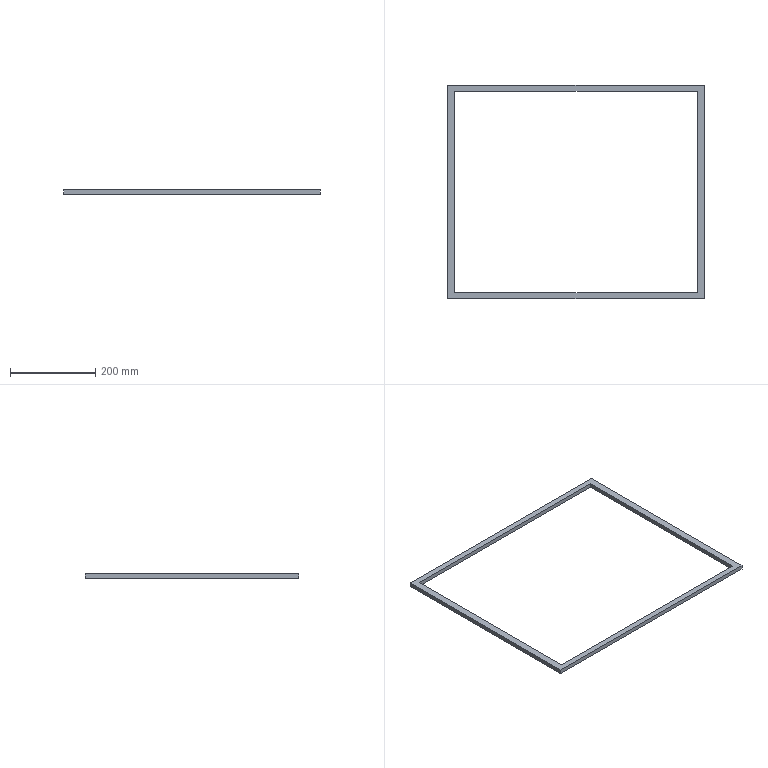Part | SolidWorks | features Extrusion 1 | 1 solid | 10 faces | box 600 x 500 x 10 mm | volume 317236 mm3 | plane 10
STEP:
#1=CARTESIAN_POINT('',(300.,-250.,10.));
#2=VERTEX_POINT('',#1);
#3=CARTESIAN_POINT('',(300.,250.,10.));
#4=VERTEX_POINT('',#3);
#5=CARTESIAN_POINT('',(300.,250.,10.));
#6=DIRECTION('',(0.,1.,0.));
#7=VECTOR('',#6,1000.);
#8=LINE('',#5,#7);
#9=EDGE_CURVE('',#2,#4,#8,.T.);
#10=ORIENTED_EDGE('',*,*,#9,.T.);
#11=CARTESIAN_POINT('',(-300.,250.,10.));
#12=VERTEX_POINT('',#11);
#13=CARTESIAN_POINT('',(-300.,250.,10.));
#14=DIRECTION('',(-1.,0.,0.));
#15=VECTOR('',#14,1000.);
#16=LINE('',#13,#15);
#17=EDGE_CURVE('',#4,#12,#16,.T.);
#18=ORIENTED_EDGE('',*,*,#17,.T.);
#19=CARTESIAN_POINT('',(-300.,-250.,10.));
#20=VERTEX_POINT('',#19);
#21=CARTESIAN_POINT('',(-300.,250.,10.));
#22=DIRECTION('',(0.,-1.,0.));
#23=VECTOR('',#22,1000.);
#24=LINE('',#21,#23);
#25=EDGE_CURVE('',#12,#20,#24,.T.);
#26=ORIENTED_EDGE('',*,*,#25,.T.);
#27=CARTESIAN_POINT('',(-300.,-250.,10.));
#28=DIRECTION('',(1.,0.,0.));
#29=VECTOR('',#28,1000.);
#30=LINE('',#27,#29);
#31=EDGE_CURVE('',#20,#2,#30,.T.);
#32=ORIENTED_EDGE('',*,*,#31,.T.);
#33=EDGE_LOOP('',(#10,#18,#26,#32));
#34=FACE_OUTER_BOUND('',#33,.T.);
#35=CARTESIAN_POINT('',(283.695,236.413,10.));
#36=VERTEX_POINT('',#35);
#37=CARTESIAN_POINT('',(-283.695,236.413,10.));
#38=VERTEX_POINT('',#37);
#39=CARTESIAN_POINT('',(-283.695,236.413,10.));
#40=DIRECTION('',(-1.,0.,0.));
#41=VECTOR('',#40,1000.);
#42=LINE('',#39,#41);
#43=EDGE_CURVE('',#36,#38,#42,.T.);
#44=ORIENTED_EDGE('',*,*,#43,.F.);
#45=CARTESIAN_POINT('',(283.695,-236.413,10.));
#46=VERTEX_POINT('',#45);
#47=CARTESIAN_POINT('',(283.695,236.413,10.));
#48=DIRECTION('',(0.,1.,0.));
#49=VECTOR('',#48,1000.);
#50=LINE('',#47,#49);
#51=EDGE_CURVE('',#46,#36,#50,.T.);
#52=ORIENTED_EDGE('',*,*,#51,.F.);
#53=CARTESIAN_POINT('',(-283.695,-236.413,10.));
#54=VERTEX_POINT('',#53);
#55=CARTESIAN_POINT('',(-283.695,-236.413,10.));
#56=DIRECTION('',(1.,0.,0.));
#57=VECTOR('',#56,1000.);
#58=LINE('',#55,#57);
#59=EDGE_CURVE('',#54,#46,#58,.T.);
#60=ORIENTED_EDGE('',*,*,#59,.F.);
#61=CARTESIAN_POINT('',(-283.695,236.413,10.));
#62=DIRECTION('',(0.,-1.,0.));
#63=VECTOR('',#62,1000.);
#64=LINE('',#61,#63);
#65=EDGE_CURVE('',#38,#54,#64,.T.);
#66=ORIENTED_EDGE('',*,*,#65,.F.);
#67=EDGE_LOOP('',(#44,#52,#60,#66));
#68=FACE_BOUND('',#67,.T.);
#69=CARTESIAN_POINT('',(0.,0.,10.));
#70=DIRECTION('',(0.,0.,1.));
#71=DIRECTION('',(1.,0.,0.));
#72=AXIS2_PLACEMENT_3D('',#69,#70,#71);
#73=PLANE('',#72);
#74=ADVANCED_FACE('',(#34,#68),#73,.T.);
#75=CARTESIAN_POINT('',(300.,-250.,0.));
#76=VERTEX_POINT('',#75);
#77=CARTESIAN_POINT('',(300.,250.,0.));
#78=VERTEX_POINT('',#77);
#79=CARTESIAN_POINT('',(300.,250.,0.));
#80=DIRECTION('',(0.,1.,0.));
#81=VECTOR('',#80,1000.);
#82=LINE('',#79,#81);
#83=EDGE_CURVE('',#76,#78,#82,.T.);
#84=ORIENTED_EDGE('',*,*,#83,.F.);
#85=CARTESIAN_POINT('',(-300.,-250.,0.));
#86=VERTEX_POINT('',#85);
#87=CARTESIAN_POINT('',(-300.,-250.,0.));
#88=DIRECTION('',(1.,0.,0.));
#89=VECTOR('',#88,1000.);
#90=LINE('',#87,#89);
#91=EDGE_CURVE('',#86,#76,#90,.T.);
#92=ORIENTED_EDGE('',*,*,#91,.F.);
#93=CARTESIAN_POINT('',(-300.,250.,0.));
#94=VERTEX_POINT('',#93);
#95=CARTESIAN_POINT('',(-300.,250.,0.));
#96=DIRECTION('',(0.,-1.,0.));
#97=VECTOR('',#96,1000.);
#98=LINE('',#95,#97);
#99=EDGE_CURVE('',#94,#86,#98,.T.);
#100=ORIENTED_EDGE('',*,*,#99,.F.);
#101=CARTESIAN_POINT('',(-300.,250.,0.));
#102=DIRECTION('',(-1.,0.,0.));
#103=VECTOR('',#102,1000.);
#104=LINE('',#101,#103);
#105=EDGE_CURVE('',#78,#94,#104,.T.);
#106=ORIENTED_EDGE('',*,*,#105,.F.);
#107=EDGE_LOOP('',(#84,#92,#100,#106));
#108=FACE_OUTER_BOUND('',#107,.T.);
#109=CARTESIAN_POINT('',(283.695,-236.413,0.));
#110=VERTEX_POINT('',#109);
#111=CARTESIAN_POINT('',(283.695,236.413,0.));
#112=VERTEX_POINT('',#111);
#113=CARTESIAN_POINT('',(283.695,236.413,0.));
#114=DIRECTION('',(0.,1.,0.));
#115=VECTOR('',#114,1000.);
#116=LINE('',#113,#115);
#117=EDGE_CURVE('',#110,#112,#116,.T.);
#118=ORIENTED_EDGE('',*,*,#117,.T.);
#119=CARTESIAN_POINT('',(-283.695,236.413,0.));
#120=VERTEX_POINT('',#119);
#121=CARTESIAN_POINT('',(-283.695,236.413,0.));
#122=DIRECTION('',(-1.,0.,0.));
#123=VECTOR('',#122,1000.);
#124=LINE('',#121,#123);
#125=EDGE_CURVE('',#112,#120,#124,.T.);
#126=ORIENTED_EDGE('',*,*,#125,.T.);
#127=CARTESIAN_POINT('',(-283.695,-236.413,0.));
#128=VERTEX_POINT('',#127);
#129=CARTESIAN_POINT('',(-283.695,236.413,0.));
#130=DIRECTION('',(0.,-1.,0.));
#131=VECTOR('',#130,1000.);
#132=LINE('',#129,#131);
#133=EDGE_CURVE('',#120,#128,#132,.T.);
#134=ORIENTED_EDGE('',*,*,#133,.T.);
#135=CARTESIAN_POINT('',(-283.695,-236.413,0.));
#136=DIRECTION('',(1.,0.,0.));
#137=VECTOR('',#136,1000.);
#138=LINE('',#135,#137);
#139=EDGE_CURVE('',#128,#110,#138,.T.);
#140=ORIENTED_EDGE('',*,*,#139,.T.);
#141=EDGE_LOOP('',(#118,#126,#134,#140));
#142=FACE_BOUND('',#141,.T.);
#143=CARTESIAN_POINT('',(0.,0.,0.));
#144=DIRECTION('',(0.,0.,1.));
#145=DIRECTION('',(1.,0.,0.));
#146=AXIS2_PLACEMENT_3D('',#143,#144,#145);
#147=PLANE('',#146);
#148=ADVANCED_FACE('',(#108,#142),#147,.F.);
#149=ORIENTED_EDGE('',*,*,#83,.T.);
#150=CARTESIAN_POINT('',(300.,250.,10.));
#151=DIRECTION('',(0.,0.,-1.));
#152=VECTOR('',#151,1000.);
#153=LINE('',#150,#152);
#154=EDGE_CURVE('',#4,#78,#153,.T.);
#155=ORIENTED_EDGE('',*,*,#154,.F.);
#156=ORIENTED_EDGE('',*,*,#9,.F.);
#157=CARTESIAN_POINT('',(300.,-250.,10.));
#158=DIRECTION('',(0.,0.,-1.));
#159=VECTOR('',#158,1000.);
#160=LINE('',#157,#159);
#161=EDGE_CURVE('',#2,#76,#160,.T.);
#162=ORIENTED_EDGE('',*,*,#161,.T.);
#163=EDGE_LOOP('',(#149,#155,#156,#162));
#164=FACE_OUTER_BOUND('',#163,.T.);
#165=CARTESIAN_POINT('',(300.,250.,10.));
#166=DIRECTION('',(-1.,0.,0.));
#167=DIRECTION('',(0.,-1.,0.));
#168=AXIS2_PLACEMENT_3D('',#165,#166,#167);
#169=PLANE('',#168);
#170=ADVANCED_FACE('',(#164),#169,.F.);
#171=ORIENTED_EDGE('',*,*,#105,.T.);
#172=CARTESIAN_POINT('',(-300.,250.,10.));
#173=DIRECTION('',(0.,0.,-1.));
#174=VECTOR('',#173,1000.);
#175=LINE('',#172,#174);
#176=EDGE_CURVE('',#12,#94,#175,.T.);
#177=ORIENTED_EDGE('',*,*,#176,.F.);
#178=ORIENTED_EDGE('',*,*,#17,.F.);
#179=ORIENTED_EDGE('',*,*,#154,.T.);
#180=EDGE_LOOP('',(#171,#177,#178,#179));
#181=FACE_OUTER_BOUND('',#180,.T.);
#182=CARTESIAN_POINT('',(-300.,250.,10.));
#183=DIRECTION('',(0.,-1.,0.));
#184=DIRECTION('',(0.,0.,-1.));
#185=AXIS2_PLACEMENT_3D('',#182,#183,#184);
#186=PLANE('',#185);
#187=ADVANCED_FACE('',(#181),#186,.F.);
#188=ORIENTED_EDGE('',*,*,#99,.T.);
#189=CARTESIAN_POINT('',(-300.,-250.,10.));
#190=DIRECTION('',(0.,0.,-1.));
#191=VECTOR('',#190,1000.);
#192=LINE('',#189,#191);
#193=EDGE_CURVE('',#20,#86,#192,.T.);
#194=ORIENTED_EDGE('',*,*,#193,.F.);
#195=ORIENTED_EDGE('',*,*,#25,.F.);
#196=ORIENTED_EDGE('',*,*,#176,.T.);
#197=EDGE_LOOP('',(#188,#194,#195,#196));
#198=FACE_OUTER_BOUND('',#197,.T.);
#199=CARTESIAN_POINT('',(-300.,250.,10.));
#200=DIRECTION('',(1.,0.,0.));
#201=DIRECTION('',(0.,1.,0.));
#202=AXIS2_PLACEMENT_3D('',#199,#200,#201);
#203=PLANE('',#202);
#204=ADVANCED_FACE('',(#198),#203,.F.);
#205=ORIENTED_EDGE('',*,*,#91,.T.);
#206=ORIENTED_EDGE('',*,*,#161,.F.);
#207=ORIENTED_EDGE('',*,*,#31,.F.);
#208=ORIENTED_EDGE('',*,*,#193,.T.);
#209=EDGE_LOOP('',(#205,#206,#207,#208));
#210=FACE_OUTER_BOUND('',#209,.T.);
#211=CARTESIAN_POINT('',(-300.,-250.,10.));
#212=DIRECTION('',(0.,1.,0.));
#213=DIRECTION('',(0.,0.,1.));
#214=AXIS2_PLACEMENT_3D('',#211,#212,#213);
#215=PLANE('',#214);
#216=ADVANCED_FACE('',(#210),#215,.F.);
#217=ORIENTED_EDGE('',*,*,#117,.F.);
#218=CARTESIAN_POINT('',(283.695,-236.413,10.));
#219=DIRECTION('',(0.,0.,-1.));
#220=VECTOR('',#219,1000.);
#221=LINE('',#218,#220);
#222=EDGE_CURVE('',#46,#110,#221,.T.);
#223=ORIENTED_EDGE('',*,*,#222,.F.);
#224=ORIENTED_EDGE('',*,*,#51,.T.);
#225=CARTESIAN_POINT('',(283.695,236.413,10.));
#226=DIRECTION('',(0.,0.,-1.));
#227=VECTOR('',#226,1000.);
#228=LINE('',#225,#227);
#229=EDGE_CURVE('',#36,#112,#228,.T.);
#230=ORIENTED_EDGE('',*,*,#229,.T.);
#231=EDGE_LOOP('',(#217,#223,#224,#230));
#232=FACE_OUTER_BOUND('',#231,.T.);
#233=CARTESIAN_POINT('',(283.695,236.413,10.));
#234=DIRECTION('',(-1.,0.,0.));
#235=DIRECTION('',(0.,0.,1.));
#236=AXIS2_PLACEMENT_3D('',#233,#234,#235);
#237=PLANE('',#236);
#238=ADVANCED_FACE('',(#232),#237,.T.);
#239=ORIENTED_EDGE('',*,*,#125,.F.);
#240=ORIENTED_EDGE('',*,*,#229,.F.);
#241=ORIENTED_EDGE('',*,*,#43,.T.);
#242=CARTESIAN_POINT('',(-283.695,236.413,10.));
#243=DIRECTION('',(0.,0.,-1.));
#244=VECTOR('',#243,1000.);
#245=LINE('',#242,#244);
#246=EDGE_CURVE('',#38,#120,#245,.T.);
#247=ORIENTED_EDGE('',*,*,#246,.T.);
#248=EDGE_LOOP('',(#239,#240,#241,#247));
#249=FACE_OUTER_BOUND('',#248,.T.);
#250=CARTESIAN_POINT('',(-283.695,236.413,10.));
#251=DIRECTION('',(0.,-1.,0.));
#252=DIRECTION('',(0.,0.,-1.));
#253=AXIS2_PLACEMENT_3D('',#250,#251,#252);
#254=PLANE('',#253);
#255=ADVANCED_FACE('',(#249),#254,.T.);
#256=ORIENTED_EDGE('',*,*,#133,.F.);
#257=ORIENTED_EDGE('',*,*,#246,.F.);
#258=ORIENTED_EDGE('',*,*,#65,.T.);
#259=CARTESIAN_POINT('',(-283.695,-236.413,10.));
#260=DIRECTION('',(0.,0.,-1.));
#261=VECTOR('',#260,1000.);
#262=LINE('',#259,#261);
#263=EDGE_CURVE('',#54,#128,#262,.T.);
#264=ORIENTED_EDGE('',*,*,#263,.T.);
#265=EDGE_LOOP('',(#256,#257,#258,#264));
#266=FACE_OUTER_BOUND('',#265,.T.);
#267=CARTESIAN_POINT('',(-283.695,236.413,10.));
#268=DIRECTION('',(1.,0.,0.));
#269=DIRECTION('',(0.,0.,-1.));
#270=AXIS2_PLACEMENT_3D('',#267,#268,#269);
#271=PLANE('',#270);
#272=ADVANCED_FACE('',(#266),#271,.T.);
#273=ORIENTED_EDGE('',*,*,#139,.F.);
#274=ORIENTED_EDGE('',*,*,#263,.F.);
#275=ORIENTED_EDGE('',*,*,#59,.T.);
#276=ORIENTED_EDGE('',*,*,#222,.T.);
#277=EDGE_LOOP('',(#273,#274,#275,#276));
#278=FACE_OUTER_BOUND('',#277,.T.);
#279=CARTESIAN_POINT('',(-283.695,-236.413,10.));
#280=DIRECTION('',(0.,1.,0.));
#281=DIRECTION('',(0.,0.,1.));
#282=AXIS2_PLACEMENT_3D('',#279,#280,#281);
#283=PLANE('',#282);
#284=ADVANCED_FACE('',(#278),#283,.T.);
#285=CLOSED_SHELL('',(#74,#148,#170,#187,#204,#216,#238,#255,#272,#284));
#286=MANIFOLD_SOLID_BREP('',#285);
#287=CARTESIAN_POINT('',(0.,0.,0.));
#288=DIRECTION('',(0.,0.,1.));
#289=DIRECTION('',(1.,0.,0.));
#290=AXIS2_PLACEMENT_3D('',#287,#288,#289);
#291=(LENGTH_UNIT()NAMED_UNIT(*)SI_UNIT(.MILLI.,.METRE.));
#292=UNCERTAINTY_MEASURE_WITH_UNIT(LENGTH_MEASURE(0.00001),#291,'','');
#293=(NAMED_UNIT(*)PLANE_ANGLE_UNIT()SI_UNIT($,.RADIAN.));
#294=(NAMED_UNIT(*)SI_UNIT($,.STERADIAN.)SOLID_ANGLE_UNIT());
#295=(GEOMETRIC_REPRESENTATION_CONTEXT(3)GLOBAL_UNCERTAINTY_ASSIGNED_CONTEXT((#292))GLOBAL_UNIT_ASSIGNED_CONTEXT((#291,#293,#294))REPRESENTATION_CONTEXT('',''));
#296=ADVANCED_BREP_SHAPE_REPRESENTATION('',(#286,#290),#295);